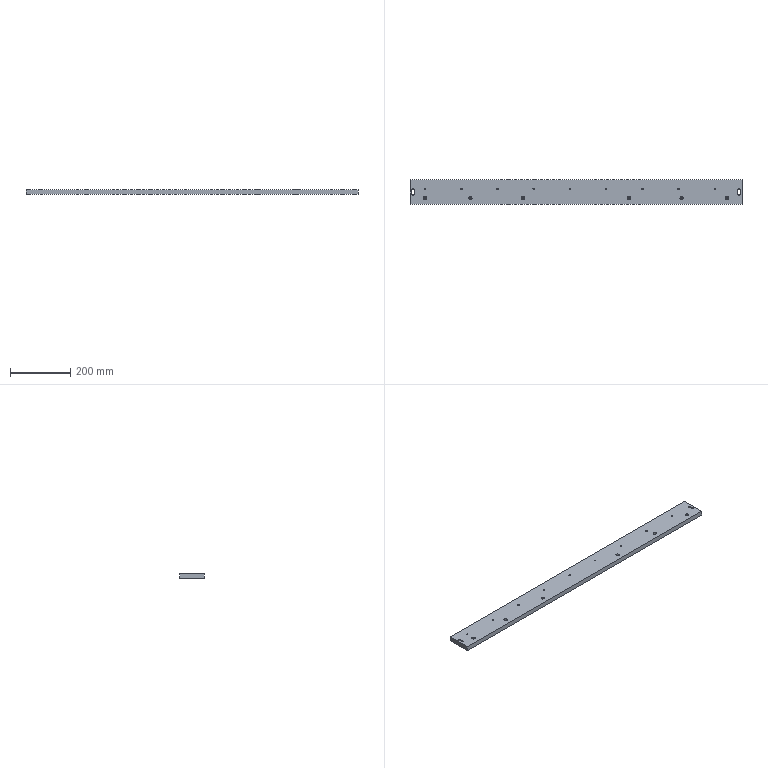Part | STEP file | 44-02-01 Guide Rail Mounting Plate A | 1 solid | 62 faces | box 1100 x 80 x 16 mm | volume 1395246 mm3 | cylinder 46 | plane 16 | commonest cylinder face diameters 5 x18 6.5 x12 11 x12 7 x4